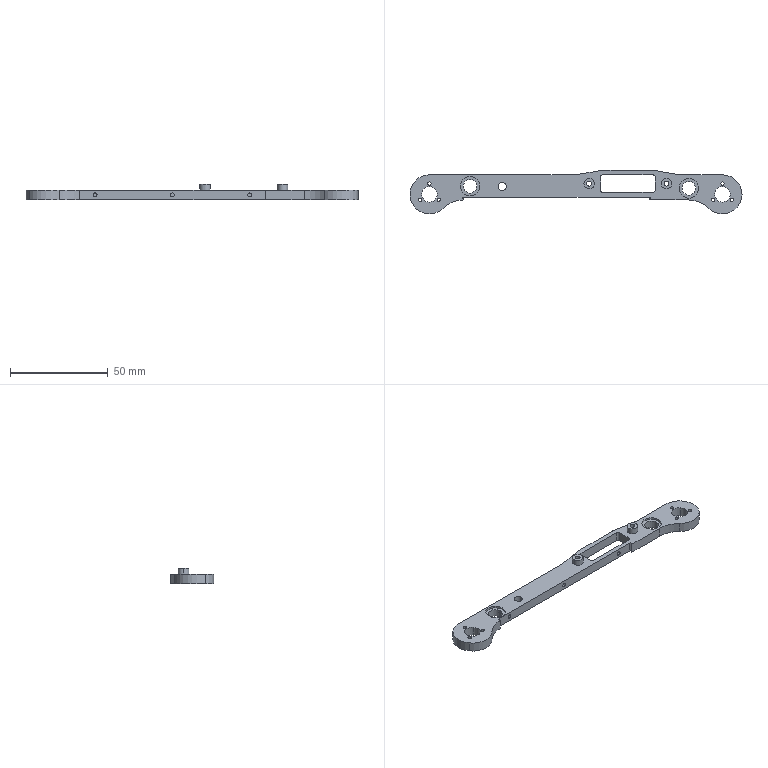Part | NX | features BREP 1 | 1 solid | 79 faces | box 170 x 22.394 x 8 mm | volume 9194 mm3 | cylinder 57 | plane 22 | commonest cylinder face diameters 1.7 x12 2 x10 10 x8 2.5 x4 5.4 x4 7 x4